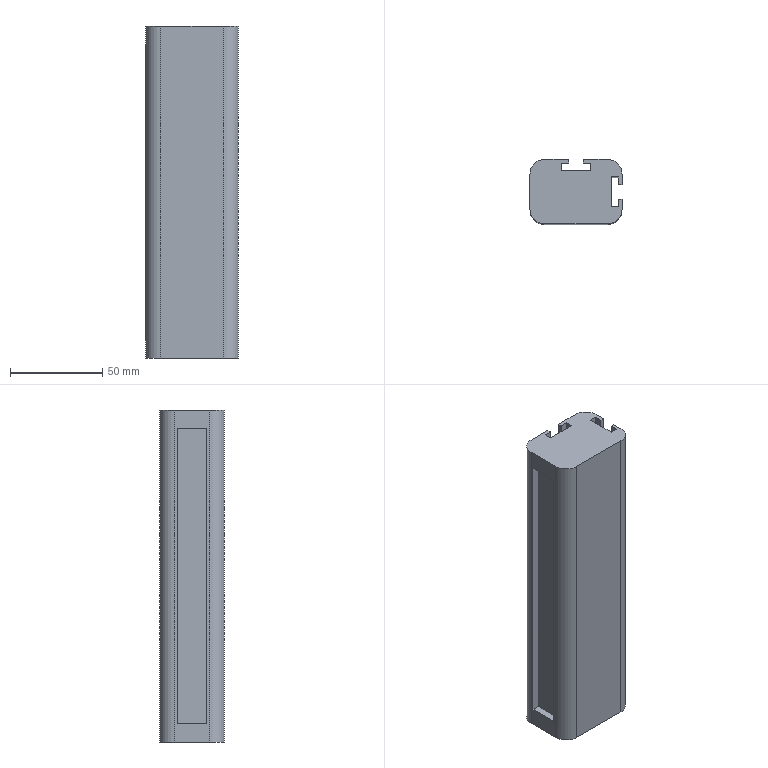Part | STEP file | light curtain sensor_Default | 1 solid | 31 faces | box 50 x 35 x 180 mm | volume 266071 mm3 | plane 27 | cylinder 4 | commonest cylinder face diameters 16 x4